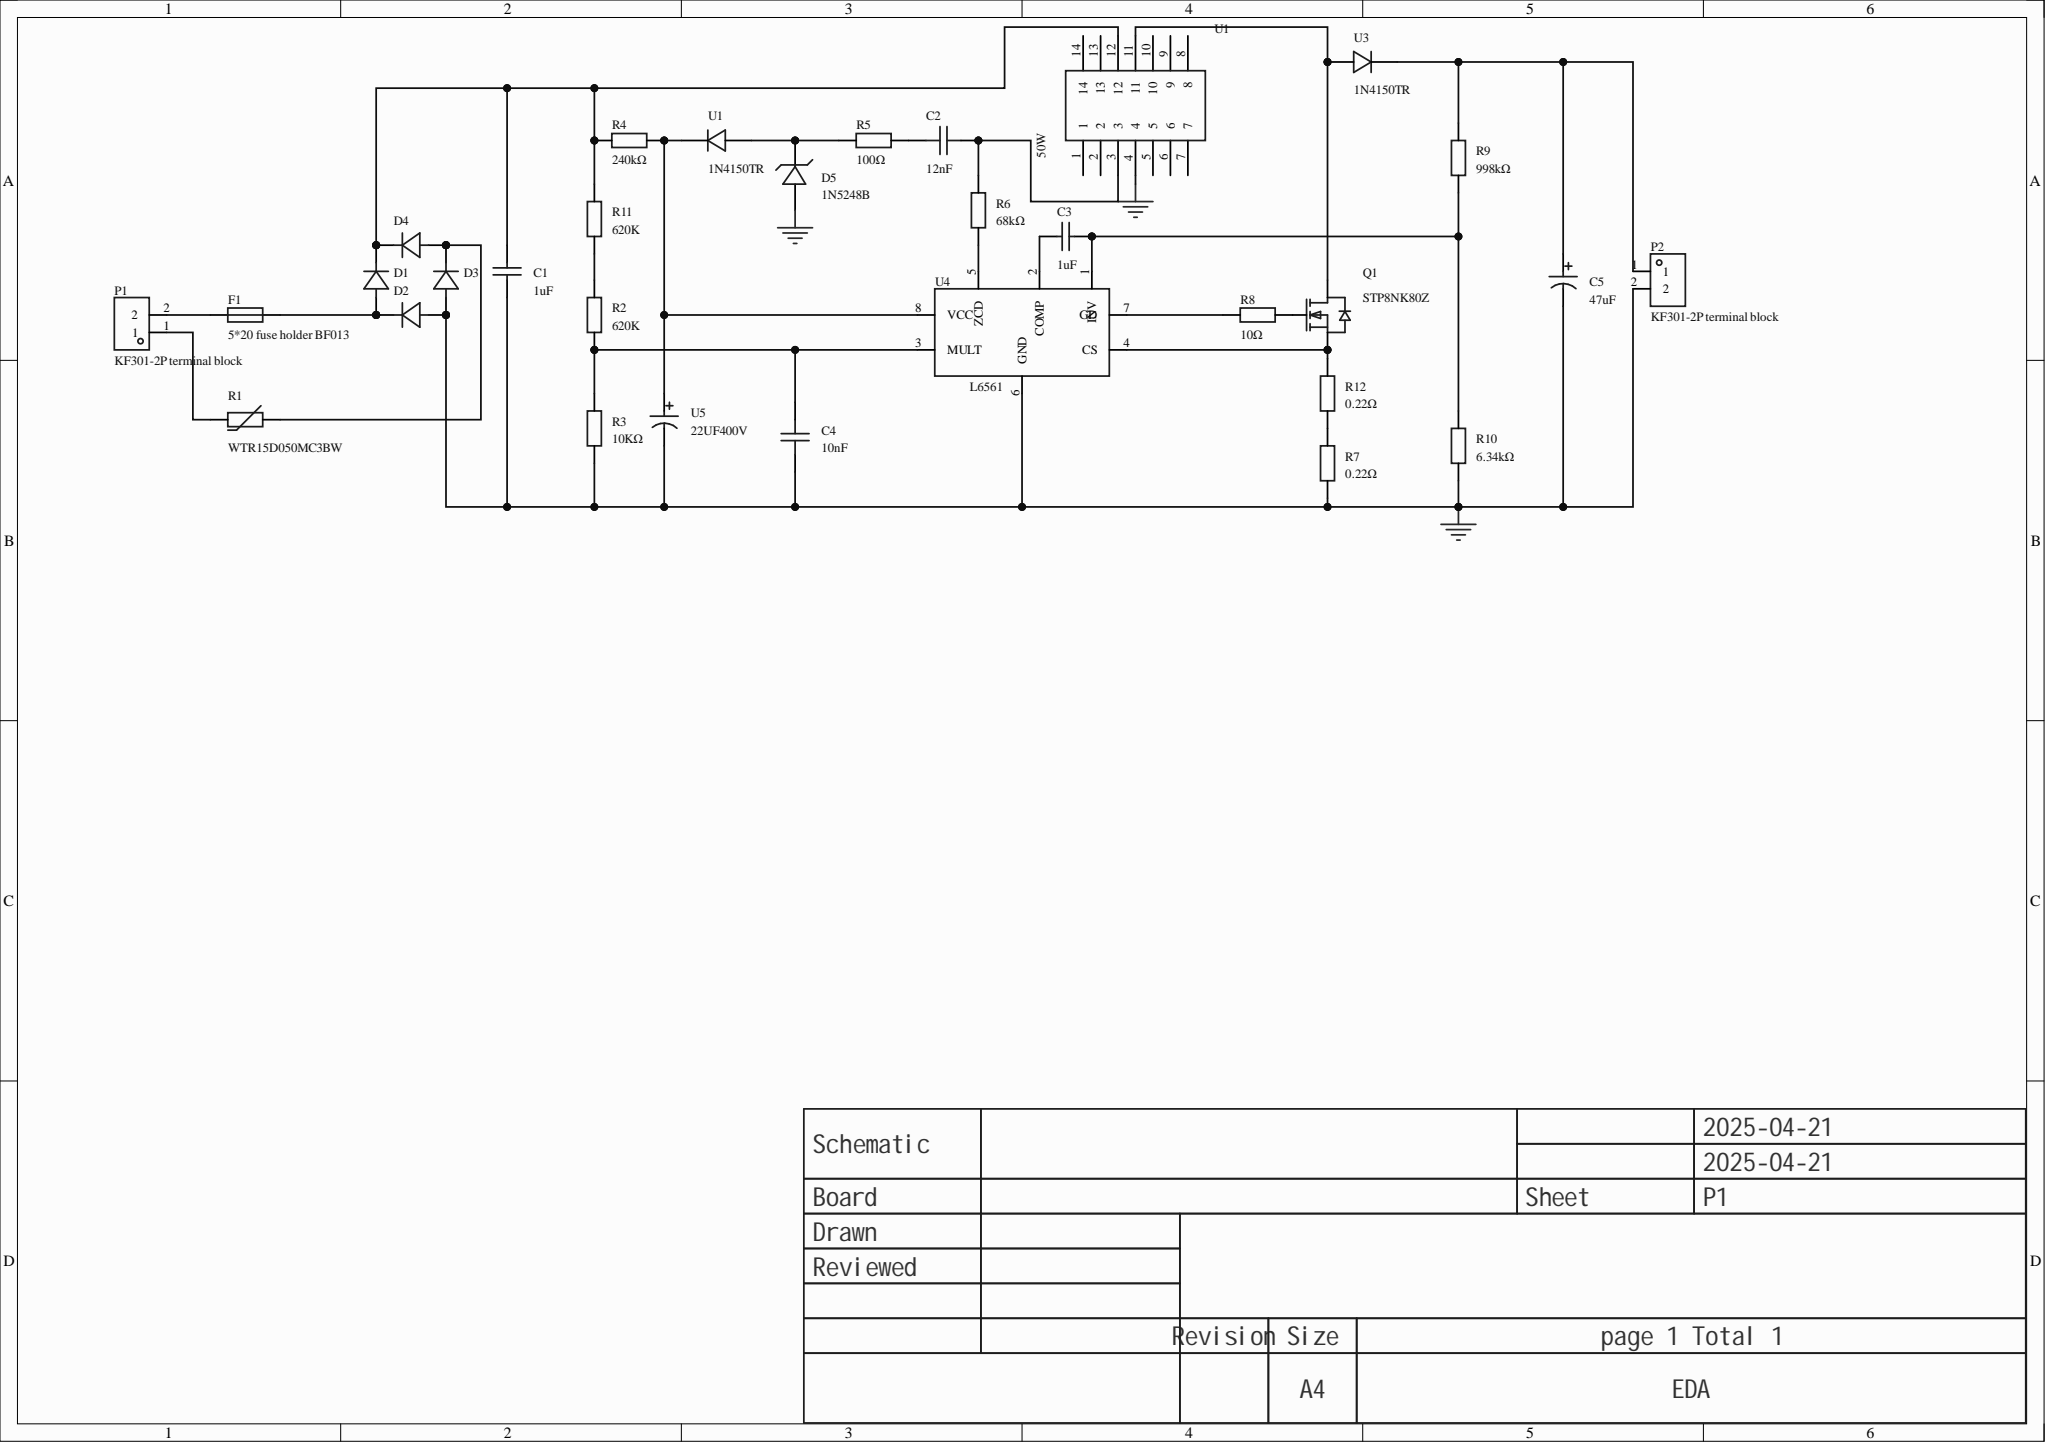Circuit board | Altium Designer | 31 parts | 21 nets
Bill of materials:
Comment,Description,Designator,Footprint,LibRef,Quantity
"1uF","Capacitance:1uF;Tolerance:±10%;Rated voltage:450V;Operating temperature:-40℃~+85℃;","C1, C3","CAP-TH_L18.0-W12.0-P15.00-D1.2","MPP105K2W1912208LC","2"
"12nF","Capacitance:12nF;Tolerance:±5%;Rated voltage:100V;Dielectric:Metallized polyester;Operating temperature:-40℃~+125℃;","C2","CAP-TH_L7.3-W4.0-P5.00-D0.5","LX2A123JD1B0070065035EOX","1"
"10nF","Capacitance:10nF;Rated voltage:1kV;Temperature coefficient:X7R;","C4","CAP-TH_L5.5-W3.5-P5.00-D1.2","C322C103JDR5TA","1"
"47uF","Capacitance:47uF;Tolerance:±20%;Rated voltage:200V;","C5","CAP-TH_BD12.5-P5.00-D0.6-FD","KM476M200J20RR0VH2FP0","1"
"","","D1, D2, D3, D4","DO_1N4007","D_1N4007A","4"
"1N5248B","Diode configuration:Single;Zener voltage(nominal):18V;Zener voltage(range):17.1V~18.9V;Power(Pd):500mW;","D5","DO-35_BD2.0-L4.2-P8.20-D0.5-RD","1N5248B","1"
"5*20 fuse holder BF013","","F1","FUSE-TH_BF013","5*20保险丝座BF013","1"
"KF301-2P terminal block","","P1, P2","CONN-TH_XY301V-A-5.0-2P","KF301-2P接线端子","2"
"STP8NK80Z","","Q1","TO-220-3_L10.0-W4.5-P2.54-L","STP8NK80Z","1"
"WTR15D050MC3BW","Resistance(25℃):-;Resistance tolerance:-;Max working voltage:-;Power:-;","R1","RES-TH_L17.5-W6.0-P7.50-D0.8-S5.20","WTR15D050MC3BW","1"
"620K","","R2, R11","Res_1/4W","Res_AXIAL-1/4W","2"
"10KΩ","","R3","Res_1/4W","Res_AXIAL-1/4W","1"
"240kΩ","","R4","Res_1/4W","Res_AXIAL-1/4W","1"
"100Ω","","R5","Res_1/4W","Res_AXIAL-1/4W","1"
"68kΩ","","R6","Res_1/4W","Res_AXIAL-1/4W","1"
"0.22Ω","","R7, R12","Res_1W","Res_AXIAL-1W","2"
"10Ω","","R8","Res_1/4W","Res_AXIAL-1/4W","1"
"998kΩ","","R9","Res_1/4W","Res_AXIAL-1/4W","1"
"6.34kΩ","","R10","Res_1/4W","Res_AXIAL-1/4W","1"
"","50W DC900V 高压高频变压器，可输出24V 50W  正负16V  0.1A 6V 0.1A .独立正16V，也可输出2A  反馈回路最大可提供15W .但是总功率不要超过50W","U1","ETD29 卧式 14脚封装","50W-900-50-24-16-06","1"
"1N4150TR","Diode configuration:Single;Forward voltage(Vf):1V@200mA;DC reverse voltage(Vr):50V;Rectified current:200mA;Reverse recovery time(trr):6ns;","U1, U3","DO-35_BD1.8-L4.1-P7.00-D0.5-RD","1N4150TR","2"
"L6561","Supply voltage:11V~18V;","U4","DIP-8_L9.8-W6.6-P2.54-LS7.6-BL","L6561","1"
"22UF400V","","U5","CAP-TH_BD8.0-P3.50-D0.6-FD","22UF400V","1"
Netlist (Protel format):
[
C1
CAP-TH_L18.0-W12.0-P15.00-D1.2
1uF



]
[
C2
CAP-TH_L7.3-W4.0-P5.00-D0.5
12nF



]
[
C3
CAP-TH_L18.0-W12.0-P15.00-D1.2
1uF



]
[
C4
CAP-TH_L5.5-W3.5-P5.00-D1.2
10nF



]
[
C5
CAP-TH_BD12.5-P5.00-D0.6-FD
47uF



]
[
D1
DO_1N4007




]
[
D2
DO_1N4007




]
[
D3
DO_1N4007




]
[
D4
DO_1N4007




]
[
D5
DO-35_BD2.0-L4.2-P8.20-D0.5-RD
1N5248B



]
[
F1
FUSE-TH_BF013
5*20 fuse holder BF013



]
[
P1
CONN-TH_XY301V-A-5.0-2P
KF301-2P terminal block



]
[
P2
CONN-TH_XY301V-A-5.0-2P
KF301-2P terminal block



]
[
Q1
TO-220-3_L10.0-W4.5-P2.54-L
STP8NK80Z



]
[
R1
RES-TH_L17.5-W6.0-P7.50-D0.8-S5.20
WTR15D050MC3BW



]
[
R2
Res_1/4W
620K



]
[
R3
Res_1/4W
10KΩ



]
[
R4
Res_1/4W
240kΩ



]
[
R5
Res_1/4W
100Ω



]
[
R6
Res_1/4W
68kΩ



]
[
R7
Res_1W
0.22Ω



]
[
R8
Res_1/4W
10Ω



]
[
R9
Res_1/4W
998kΩ



]
[
R10
Res_1/4W
6.34kΩ



]
[
R11
Res_1/4W
620K



]
[
R12
Res_1W
0.22Ω



]
[
U1
ETD29 卧式 14脚封装




]
[
U1
DO-35_BD1.8-L4.1-P7.00-D0.5-RD
1N4150TR



]
[
U3
DO-35_BD1.8-L4.1-P7.00-D0.5-RD
1N4150TR



]
[
U4
DIP-8_L9.8-W6.6-P2.54-LS7.6-BL
L6561



]
[
U5
CAP-TH_BD8.0-P3.50-D0.6-FD
22UF400V



]
(
NetR8_1
R8-1
U4-7
)
(
NetR7_2
R7-2
R12-1
)
(
NetR6_2
R6-2
U4-5
)
(
NetR4_1
R4-1
U1-1
U4-8
U5-1
)
(
NetR2_2
R2-2
R11-1
)
(
NetQ1_3
Q1-3
R12-2
U4-4
)
(
NetQ1_2
Q1-2
U1-11
U3-2
)
(
NetQ1_1
Q1-1
R8-2
)
(
NetP1_1
P1-1
R1-1
)
(
NetF1_1
F1-1
P1-2
)
(
NetD5_1
D5-1
R5-2
U1-2
)
(
NetD3_1
D3-1
D4-2
R1-2
)
(
NetD1_2
D1-2
D2-1
F1-2
)
(
NetC5_1
C5-1
P2-1
R9-1
U3-1
)
(
NetC4_2
C4-2
R2-1
R3-2
U4-3
)
(
NetC3_2
C3-2
U4-2
)
(
NetC3_1
C3-1
R9-2
R10-1
U4-1
)
(
NetC2_2
C2-2
R6-1
U1-3
)
(
NetC2_1
C2-1
R5-1
)
(
NetC1_2
C1-2
D1-1
D4-1
R4-2
R11-2
U1-12
)
(
GND
C1-1
C4-1
C5-2
D2-2
D3-2
D5-2
P2-2
R3-1
R7-1
R10-2
U1-4
U4-6
U5-2
)